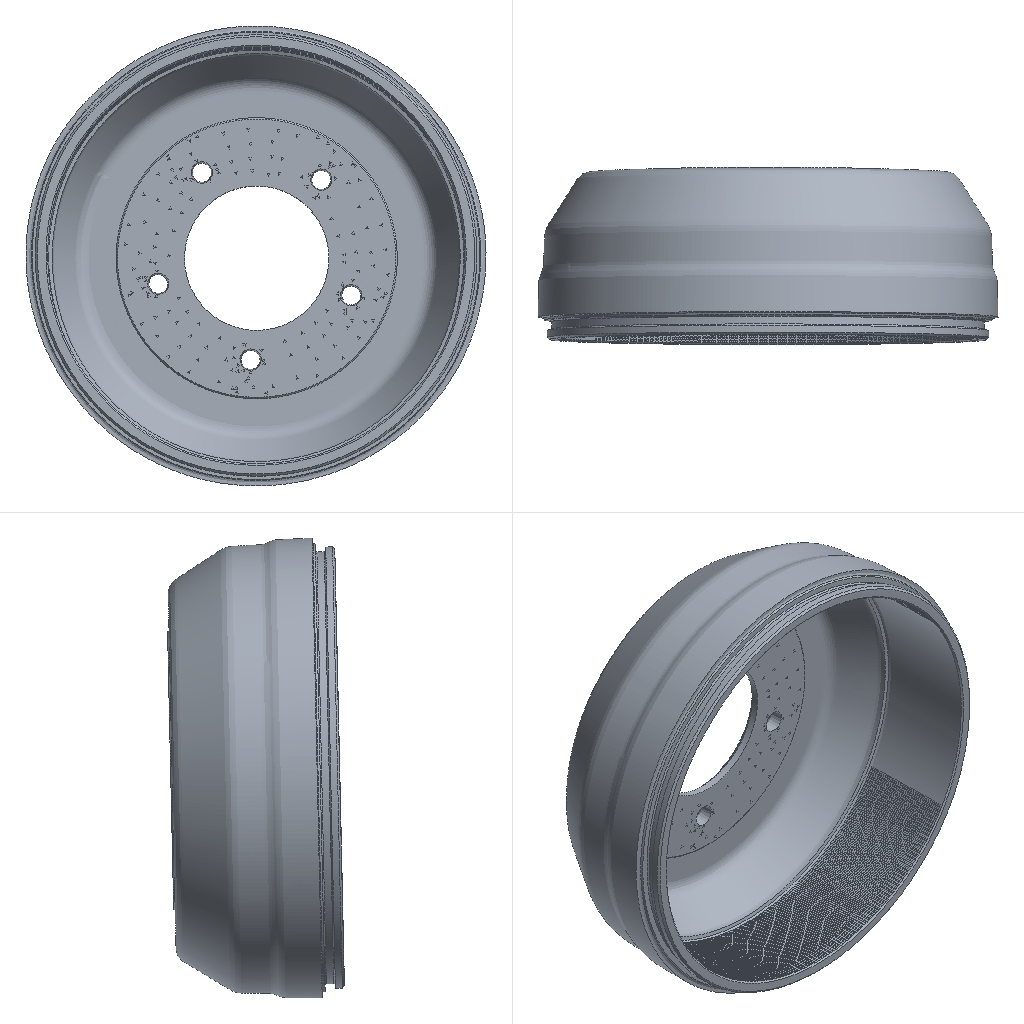Simulation study | nastran
Set-up summary:
category,name,step,type,value,unit,region
solver,nx_nastran
units,not stated in the deck,,not stated
analysis,deck,,static,static
analysis,solution,,SOL,101
load_step,SUBCASE 2,2,SUBCASE,SPC=5 LOAD=9
load_step,requested,,,1
mesh,nodes,,,160845
mesh,elements,,,6290
element_type,CHEXA,,unverified,129952
element_type,CPENTA,,unverified,4768
element_type,CQUAD4,,shell,6290
load,nodal force total,,FX,-163.68,model units
load,nodal force total,,FY,6.365,model units
load,nodal force total,,FZ,273.323,model units
load,load commands in deck,,count,12835
bc,support commands in deck,,count,1
check,setup vs results,,match,"every grid point's frame and coordinates and every element id; grid points of CHEXA, CPENTA, CQUAD4 elements"
Nastran input file, long lists of numbers shortened:
$$------------------------------------------------------------------------------$
$$                                                                              $
$$ NASTRAN Input Deck Generated by HyperMesh Version  :11.0.0.4                 $
$$ Generated using HyperMesh-Nastran Template Version : 11.0.0.47
$$                                                                              $
$$   Template:  general                                                         $
$$                                                                              $
$$------------------------------------------------------------------------------$
$$------------------------------------------------------------------------------$
$$                      Executive Control Cards                                 $
$$------------------------------------------------------------------------------$
SOL 101
CEND
$$------------------------------------------------------------------------------$
$$                      Case Control Cards                                      $
$$------------------------------------------------------------------------------$
  DISPLACEMENT = ALL
  STRAIN = ALL
  STRESS = ALL
$
$HMNAME LOADSTEP               2"Brake"
SUBCASE       2
  LABEL= Brake
  SPC =        5
  LOAD =        9
$$------------------------------------------------------------------------------$
$$                      Bulk Data Cards                                         $
$$------------------------------------------------------------------------------$
BEGIN BULK
PARAM,AUTOSPC,YES
PARAM,POST,-1
$$
$$  GRID Data
$$
GRID          87        -69.2835737.9974-331.509
GRID         330        -39.0897738.5584-305.361
$ (160843 more lines like these left out)
$$
$$  SPOINT Data
$$
$$
$$------------------------------------------------------------------------------$
$$             Group Definitions                                                $
$$------------------------------------------------------------------------------$
$$
$$ RBE2 Elements - Multiple dependent nodes
$$
RBE2      242185  167645  123456     552    5171    5172    5173    5174+
+           5175    5176    5177    5178    5179    5180    5181    5182+
+           5183    5184    5185    5186    5187    5188    5189    5190+
+           5191    5979    6002    6010    6020    6033    6034    6051+
+           6076    6107    6108    6140    6164    6193    6206    6235+
+           6241    6288    6296    6340    6341    6382    6393    6401+
+           6422    6425    6448    6453    6456    6464    6484    9334+
+           9813    9814    9815    9816    9817    9818    9819    9820+
+           9821    9822    9823    9824    9825    9826    9827    9828+
+           9829    9830    9831    9832    9833   10621   10644   10652+
+          10662   10675   10676   10693   10718   10749   10750   10782+
+          10806   10835   10848   10877   10883   10930   10938   10982+
+          10983   11024   11035   11043   11064   11067   11090   11095+
+          11098   11106   17569   17570   17571   17572   17625   17626+
+          17627   17628   17657   17658   17659   17660   17677   17678+
+          17679   17680   17737   17738   17739   17740   17841   17842+
+          17843   17844   17849   17850   17851   17852   18085   18086+
+          18087   18088   18257   18258   18259   18260   18293   18294+
+          18295   18296   18497   18498   18499   18500   18541   18542+
+          18543   18544   18709   18710   18711   18712   18921   18923+
+          18925   18927   18953   18954   18955   18956   19122   19124+
+          19126   19128   19182   19184   19186   19188   19325   19327+
+          19329   19331   19353   19355   19357   19359   19445   19447+
+          19449   19451   19477   19479   19481   19483   19530   19532+
+          19534   19536
RBE2      242186  167646  123456     514    5213    5214    5215    5216+
+           5217    5218    5219    5220    5221    5222    5223    5224+
+           5225    5226    5227    5228    5229    5230    5231    5232+
+           5233    7613    7618    7621    7630    7643    7645    7660+
+           7665    7678    7684    7712    7720    7740    7752    7781+
+           7784    7802    7810    7826    7833    7853    7864    7885+
+           7886    7904    7921    7930    9332    9855    9856    9857+
+           9858    9859    9860    9861    9862    9863    9864    9865+
+           9866    9867    9868    9869    9870    9871    9872    9873+
+           9874    9875   12255   12260   12263   12272   12285   12287+
+          12302   12307   12320   12326   12354   12362   12382   12394+
+          12423   12426   12444   12452   12468   12475   12495   12506+
+          12527   12528   12546   12563   12572   24857   24858   24859+
+          24860   24861   24862   24863   24864   24869   24870   24871+
+          24872   24905   24906   24907   24908   24957   24958   24959+
+          24960   25009   25010   25011   25012   25037   25038   25039+
+          25040   25109   25110   25111   25112   25157   25158   25159+
+          25160   25245   25246   25247   25248   25393   25394   25395+
+          25396   25409   25411   25413   25415   25549   25551   25553+
+          25555   25642   25644   25646   25648   25693   25695   25697+
+          25699   25774   25776   25778   25780   25882   25884   25886+
+          25888   25922   25924   25926   25928   26026   26028   26030+
+          26032   26045   26047   26049   26051   26121   26123   26125+
+          26127   26145   26147   26149   26151
RBE2      242187  167647  123456     499    5234    5235    5236    5237+
+           5238    5239    5240    5241    5242    5243    5244    5245+
+           5246    5247    5248    5249    5250    5251    5252    5253+
+           5254    8556    8559    8574    8606    8631    8668    8676+
+           8712    8727    8747    8789    8801    8846    8856    8899+
+           8938    8963    8971    8992    9020    9041    9042    9059+
+           9060    9066    9331    9876    9877    9878    9879    9880+
+           9881    9882    9883    9884    9885    9886    9887    9888+
+           9889    9890    9891    9892    9893    9894    9895    9896+
+          13198   13201   13216   13248   13273   13310   13318   13354+
+          13369   13389   13431   13443   13488   13498   13541   13580+
+          13605   13613   13634   13662   13683   13684   13701   13702+
+          13708   29389   29390   29391   29392   29393   29394   29395+
+          29396   29417   29418   29419   29420   29489   29490   29491+
+          29492   29529   29530   29531   29532   29641   29642   29643+
+          29644   29725   29726   29727   29728   29873   29874   29875+
+          29876   29917   29918   29919   29920   30109   30110   30111+
+          30112   30189   30190   30191   30192   30353   30354   30355+
+          30356   30409   30410   30411   30412   30573   30574   30575+
+          30576   30786   30788   30790   30792   30905   30907   30909+
+          30911   30974   30976   30978   30980   31078   31080   31082+
+          31084   31146   31148   31150   31152   31229   31231   31233+
+          31235   31238   31240   31242   31244   31289   31291   31293+
+          31295
RBE2      242188  167648  123456     477    5192    5193    5194    5195+
+           5196    5197    5198    5199    5200    5201    5202    5203+
+           5204    5205    5206    5207    5208    5209    5210    5211+
+           5212    7454    7456    7457    7458    7464    7480    7491+
+           7492    7524    7528    7564    7581    7605    7623    7635+
+           7641    7653    7664    7679    7681    7697    7698    7709+
+           7719    7733    9330    9834    9835    9836    9837    9838+
+           9839    9840    9841    9842    9843    9844    9845    9846+
+           9847    9848    9849    9850    9851    9852    9853    9854+
+          12096   12098   12099   12100   12106   12122   12133   12134+
+          12166   12170   12195   12206   12223   12247   12265   12277+
+          12283   12295   12306   12321   12323   12339   12340   12351+
+          12361   12375   24077   24078   24079   24080   24085   24086+
+          24087   24088   24089   24090   24091   24092   24113   24114+
+          24115   24116   24129   24130   24131   24132   24217   24218+
+          24219   24220   24293   24294   24295   24296   24337   24338+
+          24339   24340   24417   24418   24419   24420   24477   24478+
+          24479   24480   24557   24558   24559   24560   24629   24631+
+          24633   24635   24669   24670   24671   24672   24770   24772+
+          24774   24776   24873   24875   24877   24879   24941   24943+
+          24945   24947   25002   25004   25006   25008   25054   25056+
+          25058   25060   25126   25128   25130   25132   25146   25148+
+          25150   25152   25190   25192   25194   25196   25237   25239+
+          25241   25243
RBE2      242189  167649  123456     531    5150    5151    5152    5153+
+           5154    5155    5156    5157    5158    5159    5160    5161+
+           5162    5163    5164    5165    5166    5167    5168    5169+
+           5170    5790    5793    5814    5817    5829    5870    5874+
+           5907    5908    5951    5966    6016    6030    6069    6085+
+           6127    6163    6184    6207    6226    6252    6262    6271+
+           6284    6298    6302    6322    9333    9792    9793    9794+
+           9795    9796    9797    9798    9799    9800    9801    9802+
+           9803    9804    9805    9806    9807    9808    9809    9810+
+           9811    9812   10432   10435   10456   10459   10471   10512+
+          10516   10549   10550   10593   10608   10658   10672   10711+
+          10727   10769   10805   10826   10849   10868   10894   10904+
+          10913   10926   10940   10944   10964   16677   16678   16679+
+          16680   16681   16682   16683   16684   16733   16734   16735+
+          16736   16773   16774   16775   16776   16805   16806   16807+
+          16808   16913   16914   16915   16916   17053   17054   17055+
+          17056   17105   17106   17107   17108   17229   17230   17231+
+          17232   17441   17442   17443   17444   17489   17490   17491+
+          17492   17689   17690   17691   17692   17781   17782   17783+
+          17784   18045   18046   18047   18048   18093   18095   18097+
+          18099   18329   18331   18333   18335   18441   18443   18445+
+          18447   18586   18588   18590   18592   18638   18640   18642+
+          18644   18717   18719   18721   18723   18745   18747   18749+
+          18751   18829   18831   18833   18835
RBE2      242190  167650  123456  167645  167646  167647  167648  167649+
+
$
$HMMOVE      113
$         242185THRU      242190
$
$
$  CQUAD4 Elements
$
CQUAD4    259709       3  136762  136763  136186  136184
CQUAD4    260660       3  126321  126322  123718  123715
$ (6288 more lines like these left out)
$
$HMMOVE      239
$         259709  260660  277513  277651  277653  277655  277657  277659  277661
$         277663  277665  277667  277669  277671  277673  277675  277677  277679
$ (179 more lines like these left out)
CHEXA      17548       1   17327   17591   17463   17215   17328   17592+
+          17464   17216
CHEXA      17549       1   17328   17592   17464   17216   10643   10706+
+          10678   10623
$ (259900 more lines like these left out)
$
$HMMOVE      112
$          17548THRU       17764   17770THRU       17827   22271THRU       22325
$          35611THRU       36834   36971THRU       37106   49571THRU       49880
$ (71 more lines like these left out)
CPENTA     13610       1    5279    5306    5278   14153   14273   14145
CPENTA     13611       1   14153   14273   14145   14154   14274   14146
$ (4766 more lines like these left out)
$
$HMMOVE      112
$          13610THRU       13614   13820THRU       13824   13915THRU       13919
$          14050THRU       14054   14650THRU       14654   14850THRU       14854
$ (80 more lines like these left out)
PSHELL         3       10.001          1               1
$
$$
$$  PSOLID Data
$
$HMNAME PROP                   1"EN1-1126-AA.64" 5
$HWCOLOR PROP                  1      29
PSOLID         1       1
$$--------------------------------------------------------------
$$ HYPERMESH TAGS
$$--------------------------------------------------------------
$$BEGIN TAGS
$$END TAGS
$$
$$  MAT1 Data
$
$HMNAME MAT                    1"HT250" "MAT1"
$HWCOLOR MAT                   1       3
MAT1           1120000.0        0.27    7.8-9
$$
$$
$$
$$------------------------------------------------------------------------------$
$ (38 more lines like these left out)
LOAD           91.0         0.38       7    3.69       6
$
$$
$$  SPC Data
$$
SPC            5  167650  1234560.0
$
$$
$$  PLOAD4 Data
$$
PLOAD4         7  2810171.0
PLOAD4         7  2879591.0
PLOAD4         7  2782491.0
PLOAD4         7  2799961.0
$ (6286 more lines like these left out)
$$
$$  FORCE Data
$$
FORCE          6   54461       01.0     -.9999656.3791-4.0083936
FORCE          6  100402       01.0     -.9999656.3791-4.0083936
FORCE          6   67114       01.0     -.9999656.3791-4.0083936
FORCE          6   66726       01.0     -.9999656.3791-4.0083936
$ (6541 more lines like these left out)
ENDDATA
Results summary:
result,analysis,,,static
result,last_loadstep,,,1
result,primary field,,,displacements
result,max displacement,,,0.3291,model units